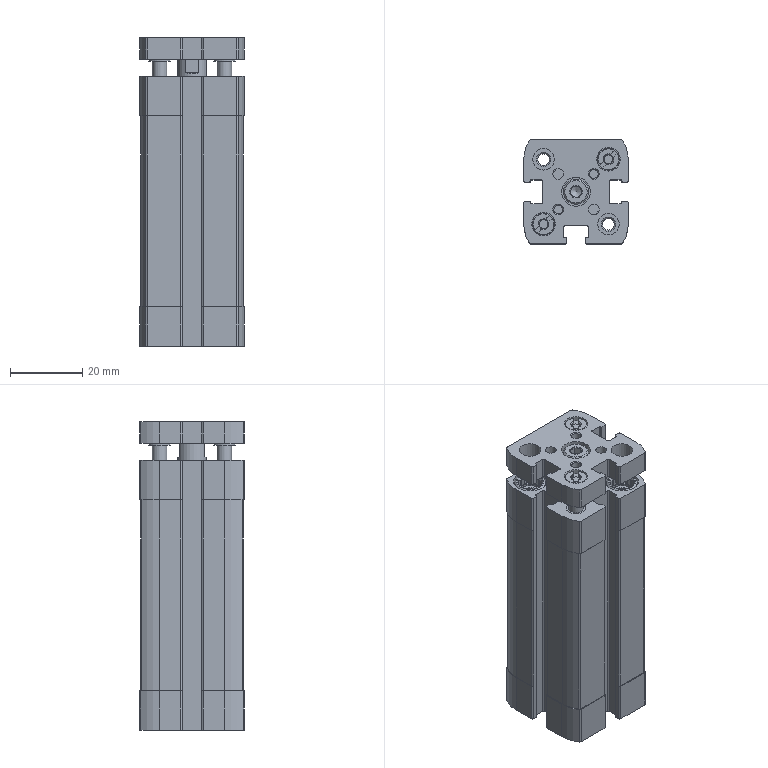Part | NX | features BREP 2 | 2 solids | 450 faces | box 29 x 29 x 85.7 mm | volume 48612 mm3 | plane 257 | cylinder 154 | cone 37 | torus 2 | commonest cylinder face diameters 0.8 x36 0.4 x24 1.2 x16 19.1 x16 6 x12 3 x7